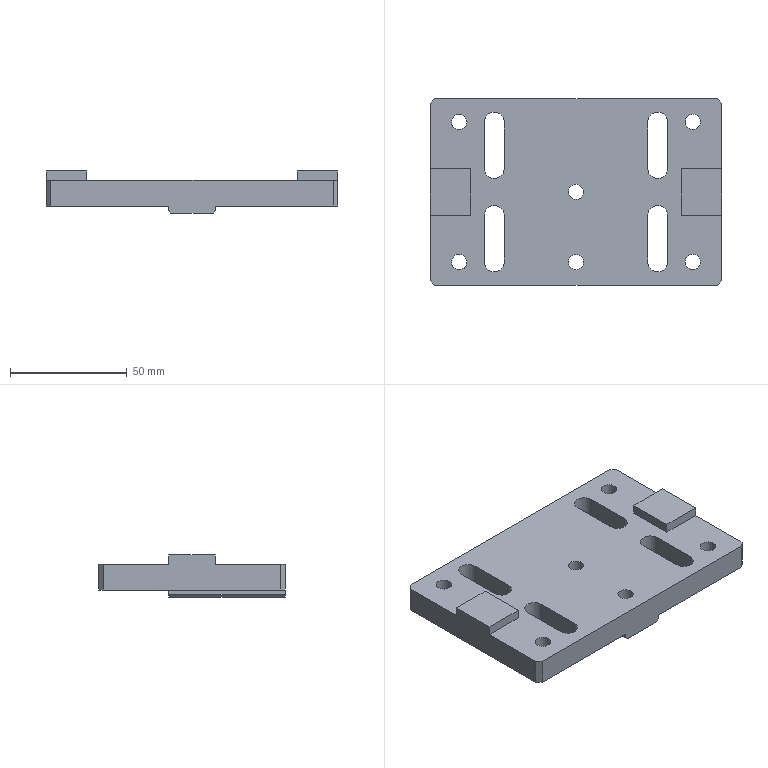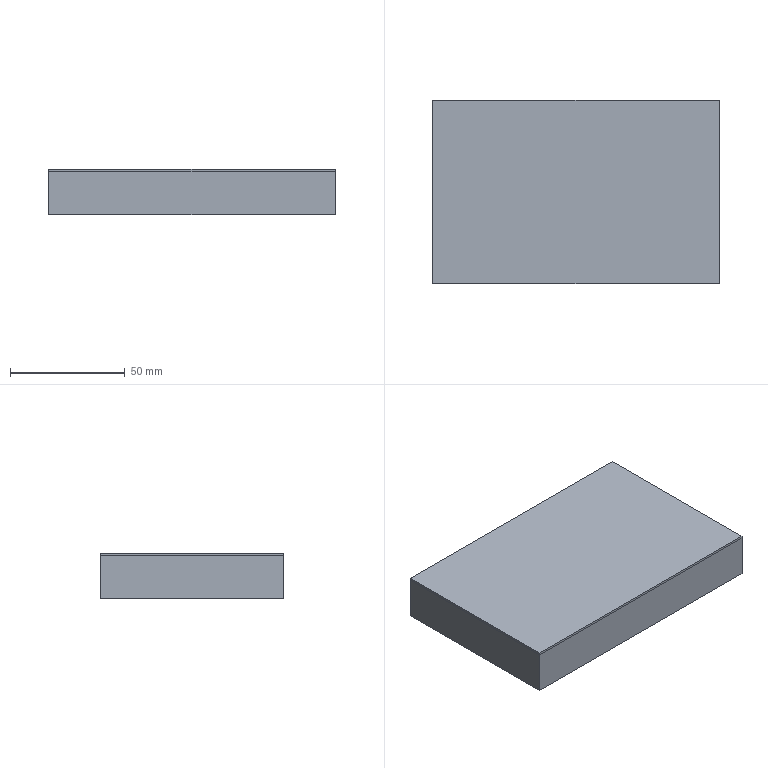CAM job | NX | 3-axis milling, drilling | part box 125 x 80 x 18 mm | stock box 125 x 80 x 20 mm
Tools:
number,name,description,diameter,corner_radius,flute_length,length,flutes
1,D63,Milling Tool-5 Parameters,63.0,0.0,50.0,75.0,2
4,D10,Milling Tool-5 Parameters,10.0,0.0,50.0,75.0,2
6,D8A45,Milling Tool-5 Parameters,8.0,0.0,50.0,75.0,2
22,6.5ZT,Drilling Tool,6.5,0.0,35.0,50.0,2
23,6.6ZT,Drilling Tool,6.6,0.0,35.0,50.0,2
2,D6,Milling Tool-5 Parameters,6.0,0.0,50.0,75.0,2
Operations:
program,operation,operation_type,tool,method,geometry_group,spindle_rpm,surface_speed,feed_per_tooth,feed_cut,feed_plunge,cut_length_mm,path_length_mm,cut_time_min,machine_time_min
1,FLOOR_WALL,VolumeBased25DMillingOperation,D63,METHOD,A,6500.0,1286.0,0.1154,1500.0,100.0,630.797,684.797,0.4205,0.4259
1,FLOOR_WALL_1,VolumeBased25DMillingOperation,D10,METHOD,A,7000.0,219.0,0.2143,3000.0,1000.0,4833.525,4947.578,1.628,1.64
1,FLOOR_WALL_1_COPY,VolumeBased25DMillingOperation,D10,METHOD,A,7000.0,219.0,0.0857,1200.0,1000.0,2261.761,2403.261,1.886,1.902
1,ZLEVEL_PROFILE_COPY,ZLevelMilling,D10,METHOD,A,7000.0,219.0,0.1429,2000.0,1000.0,349.665,996.673,0.2311,0.2958
1,DRILLING,Operation,D8A45,METHOD,A,3500.0,65.0,0.0357,250.0,0.0,38.1,416.117,0.1524,0.1902
1,DRILLING_2,Operation,6.5ZT,METHOD,A,2000.0,34.0,0.0625,250.0,0.0,40.906,174.961,0.1636,0.177
1,DRILLING_2_COPY,Operation,6.6ZT,METHOD,A,2000.0,34.0,0.0625,250.0,0.0,69.931,435.058,0.2797,0.3162
1,ZLEVEL_PROFILE_1,ZLevelMilling,D6,METHOD,A,7000.0,131.0,0.1036,1450.0,1000.0,4479.582,4941.924,3.137,3.183
1,HOLE_MILLING,CylinderMilling,D6,METHOD,A,7000.0,131.0,0.1,1400.0,100.0,911.476,1434.095,0.6511,0.7033
1,PLANAR_MILL_COPY,PlanarMilling,D8A45,METHOD,A,7000.0,1495.0,0.0893,1250.0,100.0,153.06,213.06,0.1224,0.1284
1,PLANAR_MILL_COPY_COPY,PlanarMilling,D8A45,METHOD,A,7000.0,1495.0,0.0893,1250.0,100.0,787.988,1630.043,0.6304,0.7146
2,FLOOR_WALL_COPY,VolumeBased25DMillingOperation,D63,METHOD,B,6500.0,1286.0,0.1154,1500.0,100.0,1261.594,1569.185,0.8411,0.8718
2,FLOOR_WALL_1_COPY_1,VolumeBased25DMillingOperation,D10,METHOD,B,7000.0,219.0,0.2143,3000.0,1000.0,6692.185,6889.225,2.254,2.273
2,FLOOR_WALL_1_COPY_COPY,VolumeBased25DMillingOperation,D10,METHOD,B,7000.0,219.0,0.0857,1200.0,1000.0,2538.561,2995.448,2.127,2.176
2,PLANAR_MILL_COPY_COPY_COPY,PlanarMilling,D8A45,METHOD,B,7000.0,1495.0,0.0893,1250.0,100.0,182.519,433.519,0.146,0.1711
2,PLANAR_MILL_COPY_COPY_COPY_COPY,PlanarMilling,D8A45,METHOD,B,7000.0,1495.0,0.0893,1250.0,100.0,751.399,1939.592,0.6011,0.7199